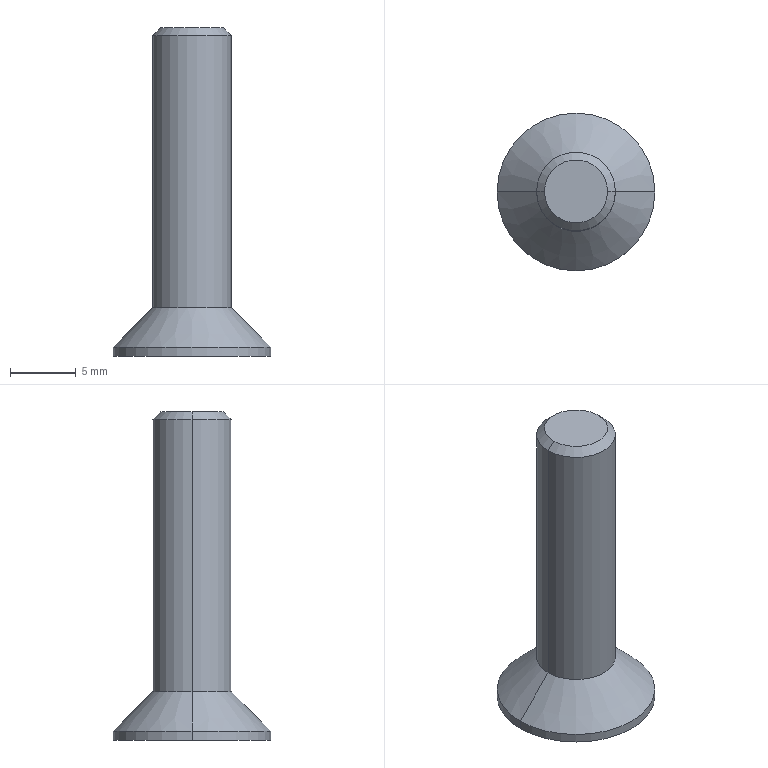Part | STEP file | LE-PJS-M6X25_PN_0009 | 1 solid | 24 faces | box 12 x 12 x 25 mm | volume 825.582 mm3 | plane 14 | cone 6 | cylinder 4 | commonest cylinder face diameters 6 x2 12 x2
STEP:
#1=CARTESIAN_POINT('',(-3.,0.,24.4));
#2=VERTEX_POINT('',#1);
#3=CARTESIAN_POINT('',(3.,0.,24.4));
#4=VERTEX_POINT('',#3);
#5=CARTESIAN_POINT('',(0.,0.,24.4));
#6=DIRECTION('',(0.,0.,-1.));
#7=DIRECTION('',(-1.,0.,0.));
#8=AXIS2_PLACEMENT_3D('',#5,#6,#7);
#9=CIRCLE('',#8,3.);
#10=EDGE_CURVE('',#2,#4,#9,.T.);
#11=ORIENTED_EDGE('',*,*,#10,.T.);
#12=CARTESIAN_POINT('',(3.,0.,3.7));
#13=VERTEX_POINT('',#12);
#14=CARTESIAN_POINT('',(3.,0.,25.));
#15=DIRECTION('',(0.,0.,-1.));
#16=VECTOR('',#15,1000.);
#17=LINE('',#14,#16);
#18=EDGE_CURVE('',#4,#13,#17,.T.);
#19=ORIENTED_EDGE('',*,*,#18,.T.);
#20=CARTESIAN_POINT('',(-3.,0.,3.7));
#21=VERTEX_POINT('',#20);
#22=CARTESIAN_POINT('',(0.,0.,3.7));
#23=DIRECTION('',(0.,0.,1.));
#24=DIRECTION('',(-1.,0.,0.));
#25=AXIS2_PLACEMENT_3D('',#22,#23,#24);
#26=CIRCLE('',#25,3.);
#27=EDGE_CURVE('',#13,#21,#26,.T.);
#28=ORIENTED_EDGE('',*,*,#27,.T.);
#29=CARTESIAN_POINT('',(-3.,0.,25.));
#30=DIRECTION('',(0.,0.,-1.));
#31=VECTOR('',#30,1000.);
#32=LINE('',#29,#31);
#33=EDGE_CURVE('',#2,#21,#32,.T.);
#34=ORIENTED_EDGE('',*,*,#33,.F.);
#35=EDGE_LOOP('',(#11,#19,#28,#34));
#36=FACE_OUTER_BOUND('',#35,.T.);
#37=CARTESIAN_POINT('',(0.,0.,25.));
#38=DIRECTION('',(0.,0.,-1.));
#39=DIRECTION('',(-1.,0.,0.));
#40=AXIS2_PLACEMENT_3D('',#37,#38,#39);
#41=CYLINDRICAL_SURFACE('',#40,3.);
#42=ADVANCED_FACE('',(#36),#41,.T.);
#43=ORIENTED_EDGE('',*,*,#27,.F.);
#44=CARTESIAN_POINT('',(6.,0.,0.7));
#45=VERTEX_POINT('',#44);
#46=CARTESIAN_POINT('',(6.,0.,0.7));
#47=DIRECTION('',(0.7071,0.,-0.7071));
#48=VECTOR('',#47,1000.);
#49=LINE('',#46,#48);
#50=EDGE_CURVE('',#13,#45,#49,.T.);
#51=ORIENTED_EDGE('',*,*,#50,.T.);
#52=CARTESIAN_POINT('',(-6.,0.,0.7));
#53=VERTEX_POINT('',#52);
#54=CARTESIAN_POINT('',(0.,0.,0.7));
#55=DIRECTION('',(0.,0.,1.));
#56=DIRECTION('',(-1.,0.,0.));
#57=AXIS2_PLACEMENT_3D('',#54,#55,#56);
#58=CIRCLE('',#57,6.);
#59=EDGE_CURVE('',#45,#53,#58,.T.);
#60=ORIENTED_EDGE('',*,*,#59,.T.);
#61=CARTESIAN_POINT('',(-6.,0.,0.7));
#62=DIRECTION('',(-0.7071,0.,-0.7071));
#63=VECTOR('',#62,1000.);
#64=LINE('',#61,#63);
#65=EDGE_CURVE('',#21,#53,#64,.T.);
#66=ORIENTED_EDGE('',*,*,#65,.F.);
#67=EDGE_LOOP('',(#43,#51,#60,#66));
#68=FACE_OUTER_BOUND('',#67,.T.);
#69=CARTESIAN_POINT('',(0.,0.,0.7));
#70=DIRECTION('',(0.,0.,-1.));
#71=DIRECTION('',(-1.,0.,0.));
#72=AXIS2_PLACEMENT_3D('',#69,#70,#71);
#73=CONICAL_SURFACE('',#72,6.,0.7854);
#74=ADVANCED_FACE('',(#68),#73,.T.);
#75=CARTESIAN_POINT('',(-2.4,0.,25.));
#76=VERTEX_POINT('',#75);
#77=CARTESIAN_POINT('',(2.4,0.,25.));
#78=VERTEX_POINT('',#77);
#79=CARTESIAN_POINT('',(0.,0.,25.));
#80=DIRECTION('',(0.,0.,-1.));
#81=DIRECTION('',(-1.,0.,0.));
#82=AXIS2_PLACEMENT_3D('',#79,#80,#81);
#83=CIRCLE('',#82,2.4);
#84=EDGE_CURVE('',#76,#78,#83,.T.);
#85=ORIENTED_EDGE('',*,*,#84,.T.);
#86=CARTESIAN_POINT('',(3.,0.,24.4));
#87=DIRECTION('',(0.7071,0.,-0.7071));
#88=VECTOR('',#87,1000.);
#89=LINE('',#86,#88);
#90=EDGE_CURVE('',#78,#4,#89,.T.);
#91=ORIENTED_EDGE('',*,*,#90,.T.);
#92=ORIENTED_EDGE('',*,*,#10,.F.);
#93=CARTESIAN_POINT('',(-3.,0.,24.4));
#94=DIRECTION('',(-0.7071,0.,-0.7071));
#95=VECTOR('',#94,1000.);
#96=LINE('',#93,#95);
#97=EDGE_CURVE('',#76,#2,#96,.T.);
#98=ORIENTED_EDGE('',*,*,#97,.F.);
#99=EDGE_LOOP('',(#85,#91,#92,#98));
#100=FACE_OUTER_BOUND('',#99,.T.);
#101=CARTESIAN_POINT('',(0.,0.,24.4));
#102=DIRECTION('',(0.,0.,-1.));
#103=DIRECTION('',(-1.,0.,0.));
#104=AXIS2_PLACEMENT_3D('',#101,#102,#103);
#105=CONICAL_SURFACE('',#104,3.,0.7854);
#106=ADVANCED_FACE('',(#100),#105,.T.);
#107=ORIENTED_EDGE('',*,*,#59,.F.);
#108=CARTESIAN_POINT('',(6.,0.,0.));
#109=VERTEX_POINT('',#108);
#110=CARTESIAN_POINT('',(6.,0.,3.7));
#111=DIRECTION('',(0.,0.,-1.));
#112=VECTOR('',#111,1000.);
#113=LINE('',#110,#112);
#114=EDGE_CURVE('',#45,#109,#113,.T.);
#115=ORIENTED_EDGE('',*,*,#114,.T.);
#116=CARTESIAN_POINT('',(-6.,0.,0.));
#117=VERTEX_POINT('',#116);
#118=CARTESIAN_POINT('',(0.,0.,0.));
#119=DIRECTION('',(0.,0.,1.));
#120=DIRECTION('',(-1.,0.,0.));
#121=AXIS2_PLACEMENT_3D('',#118,#119,#120);
#122=CIRCLE('',#121,6.);
#123=EDGE_CURVE('',#109,#117,#122,.T.);
#124=ORIENTED_EDGE('',*,*,#123,.T.);
#125=CARTESIAN_POINT('',(-6.,0.,3.7));
#126=DIRECTION('',(0.,0.,-1.));
#127=VECTOR('',#126,1000.);
#128=LINE('',#125,#127);
#129=EDGE_CURVE('',#53,#117,#128,.T.);
#130=ORIENTED_EDGE('',*,*,#129,.F.);
#131=EDGE_LOOP('',(#107,#115,#124,#130));
#132=FACE_OUTER_BOUND('',#131,.T.);
#133=CARTESIAN_POINT('',(0.,0.,3.7));
#134=DIRECTION('',(0.,0.,-1.));
#135=DIRECTION('',(-1.,0.,0.));
#136=AXIS2_PLACEMENT_3D('',#133,#134,#135);
#137=CYLINDRICAL_SURFACE('',#136,6.);
#138=ADVANCED_FACE('',(#132),#137,.T.);
#139=CARTESIAN_POINT('',(0.,0.,3.343));
#140=VERTEX_POINT('',#139);
#141=CARTESIAN_POINT('',(-2.5,0.,1.9));
#142=VERTEX_POINT('',#141);
#143=CARTESIAN_POINT('',(-2.5,0.,1.9));
#144=DIRECTION('',(-0.866,0.,-0.5));
#145=VECTOR('',#144,1000.);
#146=LINE('',#143,#145);
#147=EDGE_CURVE('',#140,#142,#146,.T.);
#148=ORIENTED_EDGE('',*,*,#147,.F.);
#149=CARTESIAN_POINT('',(2.5,0.,1.9));
#150=VERTEX_POINT('',#149);
#151=CARTESIAN_POINT('',(2.5,0.,1.9));
#152=DIRECTION('',(0.866,0.,-0.5));
#153=VECTOR('',#152,1000.);
#154=LINE('',#151,#153);
#155=EDGE_CURVE('',#140,#150,#154,.T.);
#156=ORIENTED_EDGE('',*,*,#155,.T.);
#157=CARTESIAN_POINT('',(2.165,-1.25,1.9));
#158=VERTEX_POINT('',#157);
#159=CARTESIAN_POINT('',(0.,0.,1.9));
#160=DIRECTION('',(0.,0.,1.));
#161=DIRECTION('',(-1.,0.,0.));
#162=AXIS2_PLACEMENT_3D('',#159,#160,#161);
#163=CIRCLE('',#162,2.5);
#164=EDGE_CURVE('',#158,#150,#163,.T.);
#165=ORIENTED_EDGE('',*,*,#164,.F.);
#166=CARTESIAN_POINT('',(0.,-2.5,1.9));
#167=VERTEX_POINT('',#166);
#168=CARTESIAN_POINT('',(0.,0.,1.9));
#169=DIRECTION('',(0.,0.,1.));
#170=DIRECTION('',(-1.,0.,0.));
#171=AXIS2_PLACEMENT_3D('',#168,#169,#170);
#172=CIRCLE('',#171,2.5);
#173=EDGE_CURVE('',#167,#158,#172,.T.);
#174=ORIENTED_EDGE('',*,*,#173,.F.);
#175=CARTESIAN_POINT('',(-2.165,-1.25,1.9));
#176=VERTEX_POINT('',#175);
#177=CARTESIAN_POINT('',(0.,0.,1.9));
#178=DIRECTION('',(0.,0.,1.));
#179=DIRECTION('',(-1.,0.,0.));
#180=AXIS2_PLACEMENT_3D('',#177,#178,#179);
#181=CIRCLE('',#180,2.5);
#182=EDGE_CURVE('',#176,#167,#181,.T.);
#183=ORIENTED_EDGE('',*,*,#182,.F.);
#184=CARTESIAN_POINT('',(0.,0.,1.9));
#185=DIRECTION('',(0.,0.,1.));
#186=DIRECTION('',(-1.,0.,0.));
#187=AXIS2_PLACEMENT_3D('',#184,#185,#186);
#188=CIRCLE('',#187,2.5);
#189=EDGE_CURVE('',#142,#176,#188,.T.);
#190=ORIENTED_EDGE('',*,*,#189,.F.);
#191=EDGE_LOOP('',(#148,#156,#165,#174,#183,#190));
#192=FACE_OUTER_BOUND('',#191,.T.);
#193=CARTESIAN_POINT('',(0.,0.,1.9));
#194=DIRECTION('',(0.,0.,-1.));
#195=DIRECTION('',(-1.,0.,0.));
#196=AXIS2_PLACEMENT_3D('',#193,#194,#195);
#197=CONICAL_SURFACE('',#196,2.5,1.047);
#198=ADVANCED_FACE('',(#192),#197,.F.);
#199=ORIENTED_EDGE('',*,*,#18,.F.);
#200=CARTESIAN_POINT('',(0.,0.,24.4));
#201=DIRECTION('',(0.,0.,-1.));
#202=DIRECTION('',(-1.,0.,0.));
#203=AXIS2_PLACEMENT_3D('',#200,#201,#202);
#204=CIRCLE('',#203,3.);
#205=EDGE_CURVE('',#4,#2,#204,.T.);
#206=ORIENTED_EDGE('',*,*,#205,.T.);
#207=ORIENTED_EDGE('',*,*,#33,.T.);
#208=CARTESIAN_POINT('',(0.,0.,3.7));
#209=DIRECTION('',(0.,0.,1.));
#210=DIRECTION('',(-1.,0.,0.));
#211=AXIS2_PLACEMENT_3D('',#208,#209,#210);
#212=CIRCLE('',#211,3.);
#213=EDGE_CURVE('',#21,#13,#212,.T.);
#214=ORIENTED_EDGE('',*,*,#213,.T.);
#215=EDGE_LOOP('',(#199,#206,#207,#214));
#216=FACE_OUTER_BOUND('',#215,.T.);
#217=CARTESIAN_POINT('',(0.,0.,25.));
#218=DIRECTION('',(0.,0.,-1.));
#219=DIRECTION('',(-1.,0.,0.));
#220=AXIS2_PLACEMENT_3D('',#217,#218,#219);
#221=CYLINDRICAL_SURFACE('',#220,3.);
#222=ADVANCED_FACE('',(#216),#221,.T.);
#223=ORIENTED_EDGE('',*,*,#50,.F.);
#224=ORIENTED_EDGE('',*,*,#213,.F.);
#225=ORIENTED_EDGE('',*,*,#65,.T.);
#226=CARTESIAN_POINT('',(0.,0.,0.7));
#227=DIRECTION('',(0.,0.,1.));
#228=DIRECTION('',(-1.,0.,0.));
#229=AXIS2_PLACEMENT_3D('',#226,#227,#228);
#230=CIRCLE('',#229,6.);
#231=EDGE_CURVE('',#53,#45,#230,.T.);
#232=ORIENTED_EDGE('',*,*,#231,.T.);
#233=EDGE_LOOP('',(#223,#224,#225,#232));
#234=FACE_OUTER_BOUND('',#233,.T.);
#235=CARTESIAN_POINT('',(0.,0.,0.7));
#236=DIRECTION('',(0.,0.,-1.));
#237=DIRECTION('',(-1.,0.,0.));
#238=AXIS2_PLACEMENT_3D('',#235,#236,#237);
#239=CONICAL_SURFACE('',#238,6.,0.7854);
#240=ADVANCED_FACE('',(#234),#239,.T.);
#241=ORIENTED_EDGE('',*,*,#90,.F.);
#242=CARTESIAN_POINT('',(0.,0.,25.));
#243=DIRECTION('',(0.,0.,-1.));
#244=DIRECTION('',(-1.,0.,0.));
#245=AXIS2_PLACEMENT_3D('',#242,#243,#244);
#246=CIRCLE('',#245,2.4);
#247=EDGE_CURVE('',#78,#76,#246,.T.);
#248=ORIENTED_EDGE('',*,*,#247,.T.);
#249=ORIENTED_EDGE('',*,*,#97,.T.);
#250=ORIENTED_EDGE('',*,*,#205,.F.);
#251=EDGE_LOOP('',(#241,#248,#249,#250));
#252=FACE_OUTER_BOUND('',#251,.T.);
#253=CARTESIAN_POINT('',(0.,0.,24.4));
#254=DIRECTION('',(0.,0.,-1.));
#255=DIRECTION('',(-1.,0.,0.));
#256=AXIS2_PLACEMENT_3D('',#253,#254,#255);
#257=CONICAL_SURFACE('',#256,3.,0.7854);
#258=ADVANCED_FACE('',(#252),#257,.T.);
#259=ORIENTED_EDGE('',*,*,#114,.F.);
#260=ORIENTED_EDGE('',*,*,#231,.F.);
#261=ORIENTED_EDGE('',*,*,#129,.T.);
#262=CARTESIAN_POINT('',(0.,0.,0.));
#263=DIRECTION('',(0.,0.,1.));
#264=DIRECTION('',(-1.,0.,0.));
#265=AXIS2_PLACEMENT_3D('',#262,#263,#264);
#266=CIRCLE('',#265,6.);
#267=EDGE_CURVE('',#117,#109,#266,.T.);
#268=ORIENTED_EDGE('',*,*,#267,.T.);
#269=EDGE_LOOP('',(#259,#260,#261,#268));
#270=FACE_OUTER_BOUND('',#269,.T.);
#271=CARTESIAN_POINT('',(0.,0.,3.7));
#272=DIRECTION('',(0.,0.,-1.));
#273=DIRECTION('',(-1.,0.,0.));
#274=AXIS2_PLACEMENT_3D('',#271,#272,#273);
#275=CYLINDRICAL_SURFACE('',#274,6.);
#276=ADVANCED_FACE('',(#270),#275,.T.);
#277=ORIENTED_EDGE('',*,*,#84,.F.);
#278=ORIENTED_EDGE('',*,*,#247,.F.);
#279=EDGE_LOOP('',(#277,#278));
#280=FACE_OUTER_BOUND('',#279,.T.);
#281=CARTESIAN_POINT('',(0.,0.,25.));
#282=DIRECTION('',(0.,0.,1.));
#283=DIRECTION('',(1.,0.,0.));
#284=AXIS2_PLACEMENT_3D('',#281,#282,#283);
#285=PLANE('',#284);
#286=ADVANCED_FACE('',(#280),#285,.T.);
#287=ORIENTED_EDGE('',*,*,#267,.F.);
#288=ORIENTED_EDGE('',*,*,#123,.F.);
#289=EDGE_LOOP('',(#287,#288));
#290=FACE_OUTER_BOUND('',#289,.T.);
#291=CARTESIAN_POINT('',(-2.887,0.,0.));
#292=VERTEX_POINT('',#291);
#293=CARTESIAN_POINT('',(-1.443,2.5,0.));
#294=VERTEX_POINT('',#293);
#295=CARTESIAN_POINT('',(-2.887,0.,0.));
#296=DIRECTION('',(0.5,0.866,0.));
#297=VECTOR('',#296,1000.);
#298=LINE('',#295,#297);
#299=EDGE_CURVE('',#292,#294,#298,.T.);
#300=ORIENTED_EDGE('',*,*,#299,.F.);
#301=CARTESIAN_POINT('',(-1.443,-2.5,0.));
#302=VERTEX_POINT('',#301);
#303=CARTESIAN_POINT('',(-1.443,-2.5,0.));
#304=DIRECTION('',(-0.5,0.866,0.));
#305=VECTOR('',#304,1000.);
#306=LINE('',#303,#305);
#307=EDGE_CURVE('',#302,#292,#306,.T.);
#308=ORIENTED_EDGE('',*,*,#307,.F.);
#309=CARTESIAN_POINT('',(1.443,-2.5,0.));
#310=VERTEX_POINT('',#309);
#311=CARTESIAN_POINT('',(0.,-2.5,0.));
#312=DIRECTION('',(-1.,0.,0.));
#313=VECTOR('',#312,1000.);
#314=LINE('',#311,#313);
#315=EDGE_CURVE('',#310,#302,#314,.T.);
#316=ORIENTED_EDGE('',*,*,#315,.F.);
#317=CARTESIAN_POINT('',(2.887,0.,0.));
#318=VERTEX_POINT('',#317);
#319=CARTESIAN_POINT('',(2.887,0.,0.));
#320=DIRECTION('',(-0.5,-0.866,0.));
#321=VECTOR('',#320,1000.);
#322=LINE('',#319,#321);
#323=EDGE_CURVE('',#318,#310,#322,.T.);
#324=ORIENTED_EDGE('',*,*,#323,.F.);
#325=CARTESIAN_POINT('',(1.443,2.5,0.));
#326=VERTEX_POINT('',#325);
#327=CARTESIAN_POINT('',(1.443,2.5,0.));
#328=DIRECTION('',(0.5,-0.866,0.));
#329=VECTOR('',#328,1000.);
#330=LINE('',#327,#329);
#331=EDGE_CURVE('',#326,#318,#330,.T.);
#332=ORIENTED_EDGE('',*,*,#331,.F.);
#333=CARTESIAN_POINT('',(0.,2.5,0.));
#334=DIRECTION('',(1.,0.,0.));
#335=VECTOR('',#334,1000.);
#336=LINE('',#333,#335);
#337=EDGE_CURVE('',#294,#326,#336,.T.);
#338=ORIENTED_EDGE('',*,*,#337,.F.);
#339=EDGE_LOOP('',(#300,#308,#316,#324,#332,#338));
#340=FACE_BOUND('',#339,.T.);
#341=CARTESIAN_POINT('',(0.,0.,0.));
#342=DIRECTION('',(0.,0.,1.));
#343=DIRECTION('',(1.,0.,0.));
#344=AXIS2_PLACEMENT_3D('',#341,#342,#343);
#345=PLANE('',#344);
#346=ADVANCED_FACE('',(#290,#340),#345,.F.);
#347=CARTESIAN_POINT('',(1.443,2.5,1.9));
#348=VERTEX_POINT('',#347);
#349=CARTESIAN_POINT('',(1.443,2.5,1.9));
#350=DIRECTION('',(0.,0.,-1.));
#351=VECTOR('',#350,1000.);
#352=LINE('',#349,#351);
#353=EDGE_CURVE('',#348,#326,#352,.T.);
#354=ORIENTED_EDGE('',*,*,#353,.F.);
#355=CARTESIAN_POINT('',(0.,2.5,1.9));
#356=VERTEX_POINT('',#355);
#357=CARTESIAN_POINT('',(0.,2.5,1.9));
#358=DIRECTION('',(1.,0.,0.));
#359=VECTOR('',#358,1000.);
#360=LINE('',#357,#359);
#361=EDGE_CURVE('',#356,#348,#360,.T.);
#362=ORIENTED_EDGE('',*,*,#361,.F.);
#363=CARTESIAN_POINT('',(-1.443,2.5,1.9));
#364=VERTEX_POINT('',#363);
#365=CARTESIAN_POINT('',(0.,2.5,1.9));
#366=DIRECTION('',(1.,0.,0.));
#367=VECTOR('',#366,1000.);
#368=LINE('',#365,#367);
#369=EDGE_CURVE('',#364,#356,#368,.T.);
#370=ORIENTED_EDGE('',*,*,#369,.F.);
#371=CARTESIAN_POINT('',(-1.443,2.5,1.9));
#372=DIRECTION('',(0.,0.,1.));
#373=VECTOR('',#372,1000.);
#374=LINE('',#371,#373);
#375=EDGE_CURVE('',#294,#364,#374,.T.);
#376=ORIENTED_EDGE('',*,*,#375,.F.);
#377=ORIENTED_EDGE('',*,*,#337,.T.);
#378=EDGE_LOOP('',(#354,#362,#370,#376,#377));
#379=FACE_OUTER_BOUND('',#378,.T.);
#380=CARTESIAN_POINT('',(-1.443,2.5,1.9));
#381=DIRECTION('',(0.,1.,0.));
#382=DIRECTION('',(0.,0.,1.));
#383=AXIS2_PLACEMENT_3D('',#380,#381,#382);
#384=PLANE('',#383);
#385=ADVANCED_FACE('',(#379),#384,.F.);
#386=ORIENTED_EDGE('',*,*,#375,.T.);
#387=CARTESIAN_POINT('',(-2.165,1.25,1.9));
#388=VERTEX_POINT('',#387);
#389=CARTESIAN_POINT('',(-2.165,1.25,1.9));
#390=DIRECTION('',(0.5,0.866,0.));
#391=VECTOR('',#390,1000.);
#392=LINE('',#389,#391);
#393=EDGE_CURVE('',#388,#364,#392,.T.);
#394=ORIENTED_EDGE('',*,*,#393,.F.);
#395=CARTESIAN_POINT('',(-2.887,0.,1.9));
#396=VERTEX_POINT('',#395);
#397=CARTESIAN_POINT('',(-2.887,0.,1.9));
#398=DIRECTION('',(0.5,0.866,0.));
#399=VECTOR('',#398,1000.);
#400=LINE('',#397,#399);
#401=EDGE_CURVE('',#396,#388,#400,.T.);
#402=ORIENTED_EDGE('',*,*,#401,.F.);
#403=CARTESIAN_POINT('',(-2.887,0.,1.9));
#404=DIRECTION('',(0.,0.,1.));
#405=VECTOR('',#404,1000.);
#406=LINE('',#403,#405);
#407=EDGE_CURVE('',#292,#396,#406,.T.);
#408=ORIENTED_EDGE('',*,*,#407,.F.);
#409=ORIENTED_EDGE('',*,*,#299,.T.);
#410=EDGE_LOOP('',(#386,#394,#402,#408,#409));
#411=FACE_OUTER_BOUND('',#410,.T.);
#412=CARTESIAN_POINT('',(-2.887,0.,1.9));
#413=DIRECTION('',(-0.866,0.5,0.));
#414=DIRECTION('',(-0.5,-0.866,0.));
#415=AXIS2_PLACEMENT_3D('',#412,#413,#414);
#416=PLANE('',#415);
#417=ADVANCED_FACE('',(#411),#416,.F.);
#418=ORIENTED_EDGE('',*,*,#407,.T.);
#419=CARTESIAN_POINT('',(-1.443,-2.5,1.9));
#420=DIRECTION('',(-0.5,0.866,0.));
#421=VECTOR('',#420,1000.);
#422=LINE('',#419,#421);
#423=EDGE_CURVE('',#176,#396,#422,.T.);
#424=ORIENTED_EDGE('',*,*,#423,.F.);
#425=CARTESIAN_POINT('',(-1.443,-2.5,1.9));
#426=VERTEX_POINT('',#425);
#427=CARTESIAN_POINT('',(-1.443,-2.5,1.9));
#428=DIRECTION('',(-0.5,0.866,0.));
#429=VECTOR('',#428,1000.);
#430=LINE('',#427,#429);
#431=EDGE_CURVE('',#426,#176,#430,.T.);
#432=ORIENTED_EDGE('',*,*,#431,.F.);
#433=CARTESIAN_POINT('',(-1.443,-2.5,1.9));
#434=DIRECTION('',(0.,0.,1.));
#435=VECTOR('',#434,1000.);
#436=LINE('',#433,#435);
#437=EDGE_CURVE('',#302,#426,#436,.T.);
#438=ORIENTED_EDGE('',*,*,#437,.F.);
#439=ORIENTED_EDGE('',*,*,#307,.T.);
#440=EDGE_LOOP('',(#418,#424,#432,#438,#439));
#441=FACE_OUTER_BOUND('',#440,.T.);
#442=CARTESIAN_POINT('',(-1.443,-2.5,1.9));
#443=DIRECTION('',(-0.866,-0.5,0.));
#444=DIRECTION('',(0.5,-0.866,0.));
#445=AXIS2_PLACEMENT_3D('',#442,#443,#444);
#446=PLANE('',#445);
#447=ADVANCED_FACE('',(#441),#446,.F.);
#448=ORIENTED_EDGE('',*,*,#437,.T.);
#449=CARTESIAN_POINT('',(0.,-2.5,1.9));
#450=DIRECTION('',(-1.,0.,0.));
#451=VECTOR('',#450,1000.);
#452=LINE('',#449,#451);
#453=EDGE_CURVE('',#167,#426,#452,.T.);
#454=ORIENTED_EDGE('',*,*,#453,.F.);
#455=CARTESIAN_POINT('',(1.443,-2.5,1.9));
#456=VERTEX_POINT('',#455);
#457=CARTESIAN_POINT('',(0.,-2.5,1.9));
#458=DIRECTION('',(-1.,0.,0.));
#459=VECTOR('',#458,1000.);
#460=LINE('',#457,#459);
#461=EDGE_CURVE('',#456,#167,#460,.T.);
#462=ORIENTED_EDGE('',*,*,#461,.F.);
#463=CARTESIAN_POINT('',(1.443,-2.5,1.9));
#464=DIRECTION('',(0.,0.,1.));
#465=VECTOR('',#464,1000.);
#466=LINE('',#463,#465);
#467=EDGE_CURVE('',#310,#456,#466,.T.);
#468=ORIENTED_EDGE('',*,*,#467,.F.);
#469=ORIENTED_EDGE('',*,*,#315,.T.);
#470=EDGE_LOOP('',(#448,#454,#462,#468,#469));
#471=FACE_OUTER_BOUND('',#470,.T.);
#472=CARTESIAN_POINT('',(1.443,-2.5,1.9));
#473=DIRECTION('',(0.,-1.,0.));
#474=DIRECTION('',(1.,0.,0.));
#475=AXIS2_PLACEMENT_3D('',#472,#473,#474);
#476=PLANE('',#475);
#477=ADVANCED_FACE('',(#471),#476,.F.);
#478=ORIENTED_EDGE('',*,*,#467,.T.);
#479=CARTESIAN_POINT('',(2.165,-1.25,1.9));
#480=DIRECTION('',(-0.5,-0.866,0.));
#481=VECTOR('',#480,1000.);
#482=LINE('',#479,#481);
#483=EDGE_CURVE('',#158,#456,#482,.T.);
#484=ORIENTED_EDGE('',*,*,#483,.F.);
#485=CARTESIAN_POINT('',(2.887,0.,1.9));
#486=VERTEX_POINT('',#485);
#487=CARTESIAN_POINT('',(2.887,0.,1.9));
#488=DIRECTION('',(-0.5,-0.866,0.));
#489=VECTOR('',#488,1000.);
#490=LINE('',#487,#489);
#491=EDGE_CURVE('',#486,#158,#490,.T.);
#492=ORIENTED_EDGE('',*,*,#491,.F.);
#493=CARTESIAN_POINT('',(2.887,0.,1.9));
#494=DIRECTION('',(0.,0.,1.));
#495=VECTOR('',#494,1000.);
#496=LINE('',#493,#495);
#497=EDGE_CURVE('',#318,#486,#496,.T.);
#498=ORIENTED_EDGE('',*,*,#497,.F.);
#499=ORIENTED_EDGE('',*,*,#323,.T.);
#500=EDGE_LOOP('',(#478,#484,#492,#498,#499));
#501=FACE_OUTER_BOUND('',#500,.T.);
#502=CARTESIAN_POINT('',(2.887,0.,1.9));
#503=DIRECTION('',(0.866,-0.5,0.));
#504=DIRECTION('',(0.5,0.866,0.));
#505=AXIS2_PLACEMENT_3D('',#502,#503,#504);
#506=PLANE('',#505);
#507=ADVANCED_FACE('',(#501),#506,.F.);
#508=ORIENTED_EDGE('',*,*,#497,.T.);
#509=CARTESIAN_POINT('',(2.165,1.25,1.9));
#510=VERTEX_POINT('',#509);
#511=CARTESIAN_POINT('',(1.443,2.5,1.9));
#512=DIRECTION('',(0.5,-0.866,0.));
#513=VECTOR('',#512,1000.);
#514=LINE('',#511,#513);
#515=EDGE_CURVE('',#510,#486,#514,.T.);
#516=ORIENTED_EDGE('',*,*,#515,.F.);
#517=CARTESIAN_POINT('',(1.443,2.5,1.9));
#518=DIRECTION('',(0.5,-0.866,0.));
#519=VECTOR('',#518,1000.);
#520=LINE('',#517,#519);
#521=EDGE_CURVE('',#348,#510,#520,.T.);
#522=ORIENTED_EDGE('',*,*,#521,.F.);
#523=ORIENTED_EDGE('',*,*,#353,.T.);
#524=ORIENTED_EDGE('',*,*,#331,.T.);
#525=EDGE_LOOP('',(#508,#516,#522,#523,#524));
#526=FACE_OUTER_BOUND('',#525,.T.);
#527=CARTESIAN_POINT('',(1.443,2.5,1.9));
#528=DIRECTION('',(0.866,0.5,0.));
#529=DIRECTION('',(-0.5,0.866,0.));
#530=AXIS2_PLACEMENT_3D('',#527,#528,#529);
#531=PLANE('',#530);
#532=ADVANCED_FACE('',(#526),#531,.F.);
#533=ORIENTED_EDGE('',*,*,#401,.T.);
#534=CARTESIAN_POINT('',(0.,0.,1.9));
#535=DIRECTION('',(0.,0.,1.));
#536=DIRECTION('',(-1.,0.,0.));
#537=AXIS2_PLACEMENT_3D('',#534,#535,#536);
#538=CIRCLE('',#537,2.5);
#539=EDGE_CURVE('',#388,#142,#538,.T.);
#540=ORIENTED_EDGE('',*,*,#539,.T.);
#541=ORIENTED_EDGE('',*,*,#189,.T.);
#542=ORIENTED_EDGE('',*,*,#423,.T.);
#543=EDGE_LOOP('',(#533,#540,#541,#542));
#544=FACE_OUTER_BOUND('',#543,.T.);
#545=CARTESIAN_POINT('',(0.,0.,1.9));
#546=DIRECTION('',(0.,0.,-1.));
#547=DIRECTION('',(-1.,0.,0.));
#548=AXIS2_PLACEMENT_3D('',#545,#546,#547);
#549=PLANE('',#548);
#550=ADVANCED_FACE('',(#544),#549,.T.);
#551=ORIENTED_EDGE('',*,*,#491,.T.);
#552=ORIENTED_EDGE('',*,*,#164,.T.);
#553=CARTESIAN_POINT('',(0.,0.,1.9));
#554=DIRECTION('',(0.,0.,1.));
#555=DIRECTION('',(-1.,0.,0.));
#556=AXIS2_PLACEMENT_3D('',#553,#554,#555);
#557=CIRCLE('',#556,2.5);
#558=EDGE_CURVE('',#150,#510,#557,.T.);
#559=ORIENTED_EDGE('',*,*,#558,.T.);
#560=ORIENTED_EDGE('',*,*,#515,.T.);
#561=EDGE_LOOP('',(#551,#552,#559,#560));
#562=FACE_OUTER_BOUND('',#561,.T.);
#563=CARTESIAN_POINT('',(0.,0.,1.9));
#564=DIRECTION('',(0.,0.,-1.));
#565=DIRECTION('',(-1.,0.,0.));
#566=AXIS2_PLACEMENT_3D('',#563,#564,#565);
#567=PLANE('',#566);
#568=ADVANCED_FACE('',(#562),#567,.T.);
#569=ORIENTED_EDGE('',*,*,#361,.T.);
#570=ORIENTED_EDGE('',*,*,#521,.T.);
#571=CARTESIAN_POINT('',(0.,0.,1.9));
#572=DIRECTION('',(0.,0.,1.));
#573=DIRECTION('',(-1.,0.,0.));
#574=AXIS2_PLACEMENT_3D('',#571,#572,#573);
#575=CIRCLE('',#574,2.5);
#576=EDGE_CURVE('',#510,#356,#575,.T.);
#577=ORIENTED_EDGE('',*,*,#576,.T.);
#578=EDGE_LOOP('',(#569,#570,#577));
#579=FACE_OUTER_BOUND('',#578,.T.);
#580=CARTESIAN_POINT('',(0.,0.,1.9));
#581=DIRECTION('',(0.,0.,-1.));
#582=DIRECTION('',(-1.,0.,0.));
#583=AXIS2_PLACEMENT_3D('',#580,#581,#582);
#584=PLANE('',#583);
#585=ADVANCED_FACE('',(#579),#584,.T.);
#586=ORIENTED_EDGE('',*,*,#155,.F.);
#587=ORIENTED_EDGE('',*,*,#147,.T.);
#588=ORIENTED_EDGE('',*,*,#539,.F.);
#589=CARTESIAN_POINT('',(0.,0.,1.9));
#590=DIRECTION('',(0.,0.,1.));
#591=DIRECTION('',(-1.,0.,0.));
#592=AXIS2_PLACEMENT_3D('',#589,#590,#591);
#593=CIRCLE('',#592,2.5);
#594=EDGE_CURVE('',#356,#388,#593,.T.);
#595=ORIENTED_EDGE('',*,*,#594,.F.);
#596=ORIENTED_EDGE('',*,*,#576,.F.);
#597=ORIENTED_EDGE('',*,*,#558,.F.);
#598=EDGE_LOOP('',(#586,#587,#588,#595,#596,#597));
#599=FACE_OUTER_BOUND('',#598,.T.);
#600=CARTESIAN_POINT('',(0.,0.,1.9));
#601=DIRECTION('',(0.,0.,-1.));
#602=DIRECTION('',(-1.,0.,0.));
#603=AXIS2_PLACEMENT_3D('',#600,#601,#602);
#604=CONICAL_SURFACE('',#603,2.5,1.047);
#605=ADVANCED_FACE('',(#599),#604,.F.);
#606=ORIENTED_EDGE('',*,*,#393,.T.);
#607=ORIENTED_EDGE('',*,*,#369,.T.);
#608=ORIENTED_EDGE('',*,*,#594,.T.);
#609=EDGE_LOOP('',(#606,#607,#608));
#610=FACE_OUTER_BOUND('',#609,.T.);
#611=CARTESIAN_POINT('',(0.,0.,1.9));
#612=DIRECTION('',(0.,0.,-1.));
#613=DIRECTION('',(-1.,0.,0.));
#614=AXIS2_PLACEMENT_3D('',#611,#612,#613);
#615=PLANE('',#614);
#616=ADVANCED_FACE('',(#610),#615,.T.);
#617=ORIENTED_EDGE('',*,*,#483,.T.);
#618=ORIENTED_EDGE('',*,*,#461,.T.);
#619=ORIENTED_EDGE('',*,*,#173,.T.);
#620=EDGE_LOOP('',(#617,#618,#619));
#621=FACE_OUTER_BOUND('',#620,.T.);
#622=CARTESIAN_POINT('',(0.,0.,1.9));
#623=DIRECTION('',(0.,0.,-1.));
#624=DIRECTION('',(-1.,0.,0.));
#625=AXIS2_PLACEMENT_3D('',#622,#623,#624);
#626=PLANE('',#625);
#627=ADVANCED_FACE('',(#621),#626,.T.);
#628=ORIENTED_EDGE('',*,*,#453,.T.);
#629=ORIENTED_EDGE('',*,*,#431,.T.);
#630=ORIENTED_EDGE('',*,*,#182,.T.);
#631=EDGE_LOOP('',(#628,#629,#630));
#632=FACE_OUTER_BOUND('',#631,.T.);
#633=CARTESIAN_POINT('',(0.,0.,1.9));
#634=DIRECTION('',(0.,0.,-1.));
#635=DIRECTION('',(-1.,0.,0.));
#636=AXIS2_PLACEMENT_3D('',#633,#634,#635);
#637=PLANE('',#636);
#638=ADVANCED_FACE('',(#632),#637,.T.);
#639=CLOSED_SHELL('',(#42,#74,#106,#138,#198,#222,#240,#258,#276,#286,#346,#385,#417,#447,#477,#507,#532,#550,#568,#585,#605,#616,#627,#638));
#640=MANIFOLD_SOLID_BREP('',#639);
#641=CARTESIAN_POINT('',(0.,0.,0.));
#642=DIRECTION('',(0.,0.,1.));
#643=DIRECTION('',(1.,0.,0.));
#644=AXIS2_PLACEMENT_3D('',#641,#642,#643);
#645=(LENGTH_UNIT()NAMED_UNIT(*)SI_UNIT(.MILLI.,.METRE.));
#646=UNCERTAINTY_MEASURE_WITH_UNIT(LENGTH_MEASURE(0.00001),#645,'','');
#647=(NAMED_UNIT(*)PLANE_ANGLE_UNIT()SI_UNIT($,.RADIAN.));
#648=(NAMED_UNIT(*)SI_UNIT($,.STERADIAN.)SOLID_ANGLE_UNIT());
#649=(GEOMETRIC_REPRESENTATION_CONTEXT(3)GLOBAL_UNCERTAINTY_ASSIGNED_CONTEXT((#646))GLOBAL_UNIT_ASSIGNED_CONTEXT((#645,#647,#648))REPRESENTATION_CONTEXT('',''));
#650=ADVANCED_BREP_SHAPE_REPRESENTATION('',(#640,#644),#649);